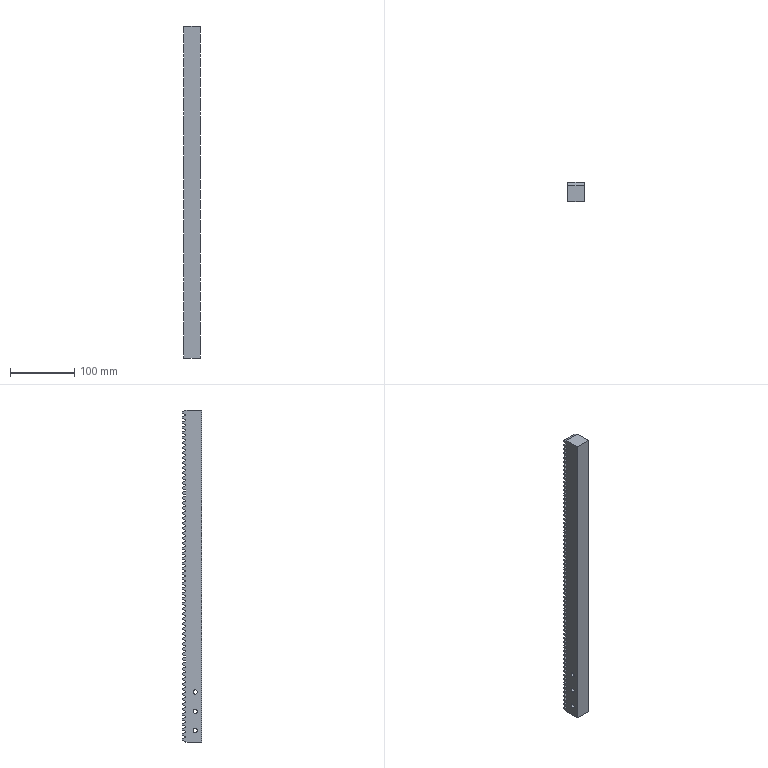Part | SolidWorks | features BaseBody 1 | 1 solid | 282 faces | box 25 x 30 x 518.364 mm | volume 351700 mm3 | plane 270 | cone 6 | cylinder 6 | commonest cylinder face diameters 6.8 x6